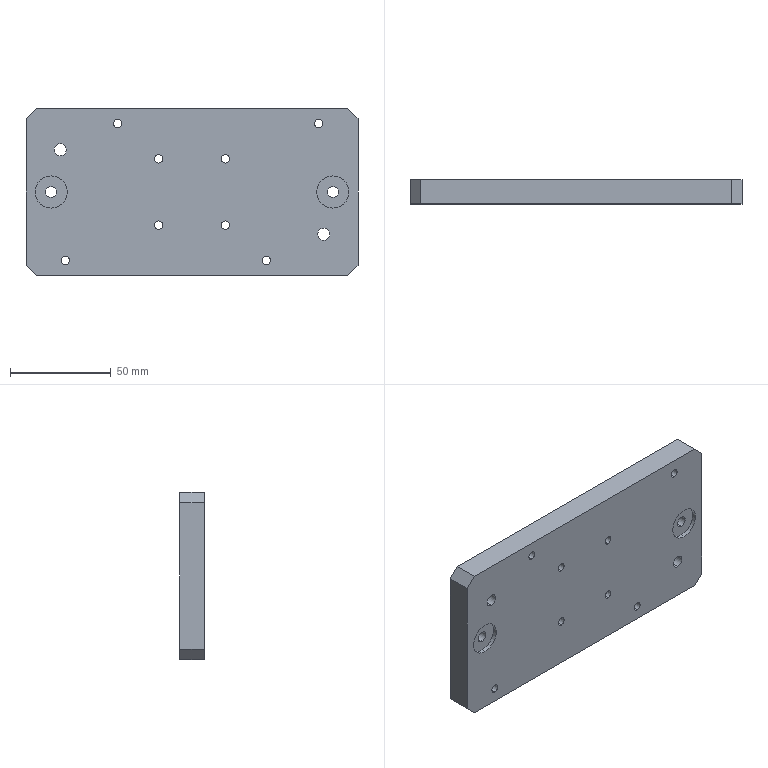Part | STEP file | PN_0056 | 1 solid | 46 faces | box 165 x 12 x 83 mm | volume 159860 mm3 | cylinder 32 | plane 14 | commonest cylinder face diameters 4.2 x16 5.5 x4 6 x4 10 x4 16 x4